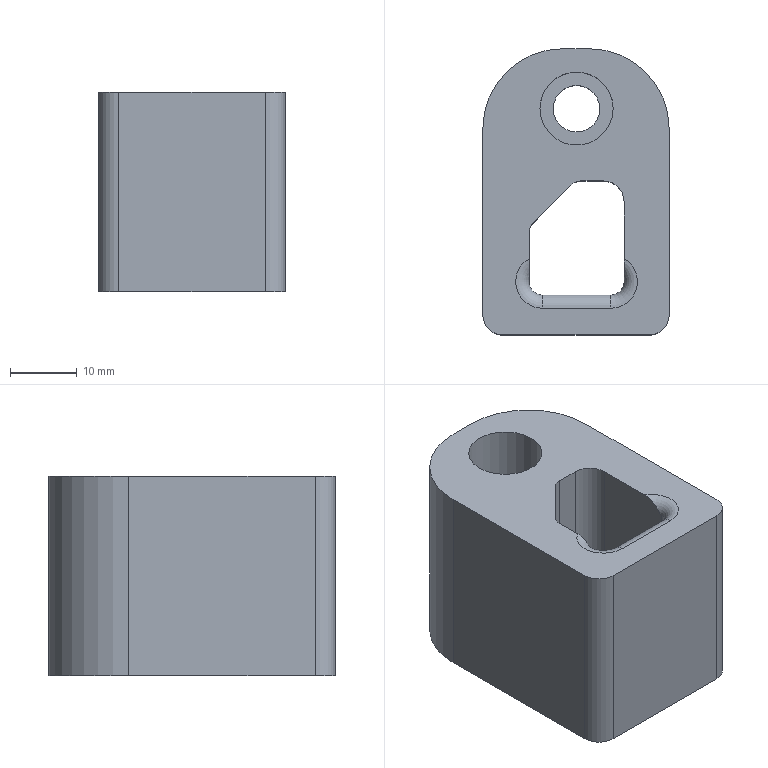Part | STEP file | 1 solid | 26 faces | box 28 x 43 x 30 mm | volume 25680 mm3 | plane 12 | cylinder 11 | torus 2 | spline 1 | commonest cylinder face diameters 4 x3 6 x2 24 x2 4.28 x1 6.28 x1 7 x1
STEP:
#1=CARTESIAN_POINT('',(-205.,-85.,-32.));
#2=VERTEX_POINT('',#1);
#3=CARTESIAN_POINT('',(-201.5,-85.,-32.));
#4=DIRECTION('',(0.,0.,-1.));
#5=DIRECTION('',(-1.,0.,0.));
#6=AXIS2_PLACEMENT_3D('',#3,#4,#5);
#7=CIRCLE('',#6,3.5);
#8=EDGE_CURVE('',#2,#2,#7,.T.);
#9=ORIENTED_EDGE('',*,*,#8,.F.);
#10=EDGE_LOOP('',(#9));
#11=FACE_BOUND('',#10,.T.);
#12=CARTESIAN_POINT('',(-212.586,-119.,-32.));
#13=VERTEX_POINT('',#12);
#14=CARTESIAN_POINT('',(-190.586,-119.,-32.));
#15=VERTEX_POINT('',#14);
#16=CARTESIAN_POINT('',(-200.586,-119.,-32.));
#17=DIRECTION('',(1.,0.,0.));
#18=VECTOR('',#17,1.);
#19=LINE('',#16,#18);
#20=EDGE_CURVE('',#13,#15,#19,.T.);
#21=ORIENTED_EDGE('',*,*,#20,.F.);
#22=CARTESIAN_POINT('',(-215.586,-116.,-32.));
#23=VERTEX_POINT('',#22);
#24=CARTESIAN_POINT('',(-212.586,-116.,-32.));
#25=DIRECTION('',(0.,0.,-1.));
#26=DIRECTION('',(-1.,0.,0.));
#27=AXIS2_PLACEMENT_3D('',#24,#25,#26);
#28=CIRCLE('',#27,3.);
#29=EDGE_CURVE('',#13,#23,#28,.T.);
#30=ORIENTED_EDGE('',*,*,#29,.T.);
#31=CARTESIAN_POINT('',(-215.586,-88.,-32.));
#32=VERTEX_POINT('',#31);
#33=CARTESIAN_POINT('',(-215.586,-98.5,-32.));
#34=DIRECTION('',(0.,-1.,0.));
#35=VECTOR('',#34,1.);
#36=LINE('',#33,#35);
#37=EDGE_CURVE('',#32,#23,#36,.T.);
#38=ORIENTED_EDGE('',*,*,#37,.F.);
#39=CARTESIAN_POINT('',(-203.586,-76.,-32.));
#40=VERTEX_POINT('',#39);
#41=CARTESIAN_POINT('',(-203.586,-88.,-32.));
#42=DIRECTION('',(0.,0.,-1.));
#43=DIRECTION('',(-1.,0.,0.));
#44=AXIS2_PLACEMENT_3D('',#41,#42,#43);
#45=CIRCLE('',#44,12.);
#46=EDGE_CURVE('',#32,#40,#45,.T.);
#47=ORIENTED_EDGE('',*,*,#46,.T.);
#48=CARTESIAN_POINT('',(-199.586,-76.,-32.));
#49=VERTEX_POINT('',#48);
#50=CARTESIAN_POINT('',(-200.586,-76.,-32.));
#51=DIRECTION('',(-1.,0.,0.));
#52=VECTOR('',#51,1.);
#53=LINE('',#50,#52);
#54=EDGE_CURVE('',#49,#40,#53,.T.);
#55=ORIENTED_EDGE('',*,*,#54,.F.);
#56=CARTESIAN_POINT('',(-187.586,-88.,-32.));
#57=VERTEX_POINT('',#56);
#58=CARTESIAN_POINT('',(-199.586,-88.,-32.));
#59=DIRECTION('',(0.,0.,-1.));
#60=DIRECTION('',(-1.,0.,0.));
#61=AXIS2_PLACEMENT_3D('',#58,#59,#60);
#62=CIRCLE('',#61,12.);
#63=EDGE_CURVE('',#49,#57,#62,.T.);
#64=ORIENTED_EDGE('',*,*,#63,.T.);
#65=CARTESIAN_POINT('',(-187.586,-116.,-32.));
#66=VERTEX_POINT('',#65);
#67=CARTESIAN_POINT('',(-187.586,-98.5,-32.));
#68=DIRECTION('',(0.,1.,0.));
#69=VECTOR('',#68,1.);
#70=LINE('',#67,#69);
#71=EDGE_CURVE('',#66,#57,#70,.T.);
#72=ORIENTED_EDGE('',*,*,#71,.F.);
#73=CARTESIAN_POINT('',(-190.586,-116.,-32.));
#74=DIRECTION('',(0.,0.,-1.));
#75=DIRECTION('',(-1.,0.,0.));
#76=AXIS2_PLACEMENT_3D('',#73,#74,#75);
#77=CIRCLE('',#76,3.);
#78=EDGE_CURVE('',#66,#15,#77,.T.);
#79=ORIENTED_EDGE('',*,*,#78,.T.);
#80=EDGE_LOOP('',(#21,#30,#38,#47,#55,#64,#72,#79));
#81=FACE_BOUND('',#80,.T.);
#82=CARTESIAN_POINT('',(-200.843,-95.86,-32.));
#83=VERTEX_POINT('',#82);
#84=CARTESIAN_POINT('',(-202.356,-96.487,-32.));
#85=VERTEX_POINT('',#84);
#86=CARTESIAN_POINT('',(-200.843,-95.86,-32.));
#87=CARTESIAN_POINT('',(-200.984,-95.86,-32.));
#88=CARTESIAN_POINT('',(-201.126,-95.874,-32.));
#89=CARTESIAN_POINT('',(-201.264,-95.901,-32.));
#90=CARTESIAN_POINT('',(-201.499,-95.949,-32.));
#91=CARTESIAN_POINT('',(-201.729,-96.037,-32.));
#92=CARTESIAN_POINT('',(-201.935,-96.159,-32.));
#93=CARTESIAN_POINT('',(-202.088,-96.25,-32.));
#94=CARTESIAN_POINT('',(-202.231,-96.361,-32.));
#95=CARTESIAN_POINT('',(-202.356,-96.487,-32.));
#96=B_SPLINE_CURVE_WITH_KNOTS('',3,(#86,#87,#88,#89,#90,#91,#92,#93,#94,#95),.UNSPECIFIED.,.F.,.F.,(4,3,3,4),(0.,0.2513,0.6822,1.),.UNSPECIFIED.);
#97=EDGE_CURVE('',#83,#85,#96,.T.);
#98=ORIENTED_EDGE('',*,*,#97,.T.);
#99=CARTESIAN_POINT('',(-208.013,-102.144,-32.));
#100=VERTEX_POINT('',#99);
#101=CARTESIAN_POINT('',(-206.771,-100.901,-32.));
#102=DIRECTION('',(-0.7071,-0.7071,0.));
#103=VECTOR('',#102,1.);
#104=LINE('',#101,#103);
#105=EDGE_CURVE('',#85,#100,#104,.T.);
#106=ORIENTED_EDGE('',*,*,#105,.T.);
#107=CARTESIAN_POINT('',(-208.64,-103.657,-32.));
#108=VERTEX_POINT('',#107);
#109=CARTESIAN_POINT('',(-206.5,-103.657,-32.));
#110=DIRECTION('',(0.,0.,1.));
#111=DIRECTION('',(-1.,0.,0.));
#112=AXIS2_PLACEMENT_3D('',#109,#110,#111);
#113=CIRCLE('',#112,2.14);
#114=EDGE_CURVE('',#100,#108,#113,.T.);
#115=ORIENTED_EDGE('',*,*,#114,.T.);
#116=CARTESIAN_POINT('',(-208.64,-111.,-32.));
#117=VERTEX_POINT('',#116);
#118=CARTESIAN_POINT('',(-208.64,-104.5,-32.));
#119=DIRECTION('',(0.,1.,0.));
#120=VECTOR('',#119,1.);
#121=LINE('',#118,#120);
#122=EDGE_CURVE('',#117,#108,#121,.T.);
#123=ORIENTED_EDGE('',*,*,#122,.F.);
#124=CARTESIAN_POINT('',(-206.64,-113.,-32.));
#125=VERTEX_POINT('',#124);
#126=CARTESIAN_POINT('',(-206.64,-111.,-32.));
#127=DIRECTION('',(0.,0.,1.));
#128=DIRECTION('',(-1.,0.,0.));
#129=AXIS2_PLACEMENT_3D('',#126,#127,#128);
#130=CIRCLE('',#129,2.);
#131=EDGE_CURVE('',#117,#125,#130,.T.);
#132=ORIENTED_EDGE('',*,*,#131,.T.);
#133=CARTESIAN_POINT('',(-196.36,-113.,-32.));
#134=VERTEX_POINT('',#133);
#135=CARTESIAN_POINT('',(-194.5,-113.,-32.));
#136=DIRECTION('',(1.,0.,0.));
#137=VECTOR('',#136,1.);
#138=LINE('',#135,#137);
#139=EDGE_CURVE('',#125,#134,#138,.T.);
#140=ORIENTED_EDGE('',*,*,#139,.T.);
#141=CARTESIAN_POINT('',(-194.36,-111.,-32.));
#142=VERTEX_POINT('',#141);
#143=CARTESIAN_POINT('',(-196.36,-111.,-32.));
#144=DIRECTION('',(0.,0.,1.));
#145=DIRECTION('',(-1.,0.,0.));
#146=AXIS2_PLACEMENT_3D('',#143,#144,#145);
#147=CIRCLE('',#146,2.);
#148=EDGE_CURVE('',#134,#142,#147,.T.);
#149=ORIENTED_EDGE('',*,*,#148,.T.);
#150=CARTESIAN_POINT('',(-194.36,-99.,-32.));
#151=VERTEX_POINT('',#150);
#152=CARTESIAN_POINT('',(-194.36,-99.,-32.));
#153=DIRECTION('',(0.,1.,0.));
#154=VECTOR('',#153,1.);
#155=LINE('',#152,#154);
#156=EDGE_CURVE('',#142,#151,#155,.T.);
#157=ORIENTED_EDGE('',*,*,#156,.T.);
#158=CARTESIAN_POINT('',(-197.5,-95.86,-32.));
#159=VERTEX_POINT('',#158);
#160=CARTESIAN_POINT('',(-197.5,-99.,-32.));
#161=DIRECTION('',(0.,0.,1.));
#162=DIRECTION('',(-1.,0.,0.));
#163=AXIS2_PLACEMENT_3D('',#160,#161,#162);
#164=CIRCLE('',#163,3.14);
#165=EDGE_CURVE('',#151,#159,#164,.T.);
#166=ORIENTED_EDGE('',*,*,#165,.T.);
#167=CARTESIAN_POINT('',(-200.843,-95.86,-32.));
#168=DIRECTION('',(-1.,0.,0.));
#169=VECTOR('',#168,1.);
#170=LINE('',#167,#169);
#171=EDGE_CURVE('',#159,#83,#170,.T.);
#172=ORIENTED_EDGE('',*,*,#171,.T.);
#173=EDGE_LOOP('',(#98,#106,#115,#123,#132,#140,#149,#157,#166,#172));
#174=FACE_BOUND('',#173,.T.);
#175=CARTESIAN_POINT('',(-201.5,-9.5,-32.));
#176=DIRECTION('',(0.,0.,-1.));
#177=DIRECTION('',(-1.,0.,0.));
#178=AXIS2_PLACEMENT_3D('',#175,#176,#177);
#179=PLANE('',#178);
#180=ADVANCED_FACE('',(#11,#81,#174),#179,.T.);
#181=CARTESIAN_POINT('',(-196.,-85.,-2.));
#182=VERTEX_POINT('',#181);
#183=CARTESIAN_POINT('',(-201.5,-85.,-2.));
#184=DIRECTION('',(0.,0.,-1.));
#185=DIRECTION('',(1.,0.,0.));
#186=AXIS2_PLACEMENT_3D('',#183,#184,#185);
#187=CIRCLE('',#186,5.5);
#188=EDGE_CURVE('',#182,#182,#187,.T.);
#189=ORIENTED_EDGE('',*,*,#188,.T.);
#190=EDGE_LOOP('',(#189));
#191=FACE_BOUND('',#190,.T.);
#192=CARTESIAN_POINT('',(-194.36,-107.536,-2.));
#193=VERTEX_POINT('',#192);
#194=CARTESIAN_POINT('',(-194.36,-99.,-2.));
#195=VERTEX_POINT('',#194);
#196=CARTESIAN_POINT('',(-194.36,129.,-2.));
#197=DIRECTION('',(0.,1.,0.));
#198=VECTOR('',#197,1.);
#199=LINE('',#196,#198);
#200=EDGE_CURVE('',#193,#195,#199,.T.);
#201=ORIENTED_EDGE('',*,*,#200,.F.);
#202=CARTESIAN_POINT('',(-196.36,-115.,-2.));
#203=VERTEX_POINT('',#202);
#204=CARTESIAN_POINT('',(-196.36,-111.,-2.));
#205=DIRECTION('',(0.,0.,-1.));
#206=DIRECTION('',(1.,0.,0.));
#207=AXIS2_PLACEMENT_3D('',#204,#205,#206);
#208=CIRCLE('',#207,4.);
#209=EDGE_CURVE('',#193,#203,#208,.T.);
#210=ORIENTED_EDGE('',*,*,#209,.T.);
#211=CARTESIAN_POINT('',(-206.64,-115.,-2.));
#212=VERTEX_POINT('',#211);
#213=CARTESIAN_POINT('',(-206.64,-115.,-2.));
#214=DIRECTION('',(-1.,0.,0.));
#215=VECTOR('',#214,1.);
#216=LINE('',#213,#215);
#217=EDGE_CURVE('',#203,#212,#216,.T.);
#218=ORIENTED_EDGE('',*,*,#217,.T.);
#219=CARTESIAN_POINT('',(-208.64,-107.536,-2.));
#220=VERTEX_POINT('',#219);
#221=CARTESIAN_POINT('',(-206.64,-111.,-2.));
#222=DIRECTION('',(0.,0.,-1.));
#223=DIRECTION('',(1.,0.,0.));
#224=AXIS2_PLACEMENT_3D('',#221,#222,#223);
#225=CIRCLE('',#224,4.);
#226=EDGE_CURVE('',#212,#220,#225,.T.);
#227=ORIENTED_EDGE('',*,*,#226,.T.);
#228=CARTESIAN_POINT('',(-208.64,-103.657,-2.));
#229=VERTEX_POINT('',#228);
#230=CARTESIAN_POINT('',(-208.64,129.,-2.));
#231=DIRECTION('',(0.,1.,0.));
#232=VECTOR('',#231,1.);
#233=LINE('',#230,#232);
#234=EDGE_CURVE('',#220,#229,#233,.T.);
#235=ORIENTED_EDGE('',*,*,#234,.T.);
#236=CARTESIAN_POINT('',(-208.013,-102.144,-2.));
#237=VERTEX_POINT('',#236);
#238=CARTESIAN_POINT('',(-206.5,-103.657,-2.));
#239=DIRECTION('',(0.,0.,1.));
#240=DIRECTION('',(1.,0.,0.));
#241=AXIS2_PLACEMENT_3D('',#238,#239,#240);
#242=CIRCLE('',#241,2.14);
#243=EDGE_CURVE('',#237,#229,#242,.T.);
#244=ORIENTED_EDGE('',*,*,#243,.F.);
#245=CARTESIAN_POINT('',(-202.356,-96.487,-2.));
#246=VERTEX_POINT('',#245);
#247=CARTESIAN_POINT('',(-128.91,-23.041,-2.));
#248=DIRECTION('',(-0.7071,-0.7071,0.));
#249=VECTOR('',#248,1.);
#250=LINE('',#247,#249);
#251=EDGE_CURVE('',#246,#237,#250,.T.);
#252=ORIENTED_EDGE('',*,*,#251,.F.);
#253=CARTESIAN_POINT('',(-200.843,-95.86,-2.));
#254=VERTEX_POINT('',#253);
#255=CARTESIAN_POINT('',(-200.843,-95.86,-2.));
#256=CARTESIAN_POINT('',(-200.984,-95.86,-2.));
#257=CARTESIAN_POINT('',(-201.126,-95.874,-2.));
#258=CARTESIAN_POINT('',(-201.264,-95.901,-2.));
#259=CARTESIAN_POINT('',(-201.499,-95.949,-2.));
#260=CARTESIAN_POINT('',(-201.729,-96.037,-2.));
#261=CARTESIAN_POINT('',(-201.935,-96.159,-2.));
#262=CARTESIAN_POINT('',(-202.088,-96.25,-2.));
#263=CARTESIAN_POINT('',(-202.231,-96.361,-2.));
#264=CARTESIAN_POINT('',(-202.356,-96.487,-2.));
#265=B_SPLINE_CURVE_WITH_KNOTS('',3,(#255,#256,#257,#258,#259,#260,#261,#262,#263,#264),.UNSPECIFIED.,.F.,.F.,(4,3,3,4),(0.,0.2513,0.6822,1.),.UNSPECIFIED.);
#266=EDGE_CURVE('',#254,#246,#265,.T.);
#267=ORIENTED_EDGE('',*,*,#266,.F.);
#268=CARTESIAN_POINT('',(-197.5,-95.86,-2.));
#269=VERTEX_POINT('',#268);
#270=CARTESIAN_POINT('',(-280.951,-95.86,-2.));
#271=DIRECTION('',(-1.,0.,0.));
#272=VECTOR('',#271,1.);
#273=LINE('',#270,#272);
#274=EDGE_CURVE('',#269,#254,#273,.T.);
#275=ORIENTED_EDGE('',*,*,#274,.F.);
#276=CARTESIAN_POINT('',(-197.5,-99.,-2.));
#277=DIRECTION('',(0.,0.,-1.));
#278=DIRECTION('',(1.,0.,0.));
#279=AXIS2_PLACEMENT_3D('',#276,#277,#278);
#280=CIRCLE('',#279,3.14);
#281=EDGE_CURVE('',#269,#195,#280,.T.);
#282=ORIENTED_EDGE('',*,*,#281,.T.);
#283=EDGE_LOOP('',(#201,#210,#218,#227,#235,#244,#252,#267,#275,#282));
#284=FACE_BOUND('',#283,.T.);
#285=CARTESIAN_POINT('',(-215.586,-116.,-2.));
#286=VERTEX_POINT('',#285);
#287=CARTESIAN_POINT('',(-215.586,-88.,-2.));
#288=VERTEX_POINT('',#287);
#289=CARTESIAN_POINT('',(-215.586,-98.5,-2.));
#290=DIRECTION('',(0.,1.,0.));
#291=VECTOR('',#290,1.);
#292=LINE('',#289,#291);
#293=EDGE_CURVE('',#286,#288,#292,.T.);
#294=ORIENTED_EDGE('',*,*,#293,.F.);
#295=CARTESIAN_POINT('',(-212.586,-119.,-2.));
#296=VERTEX_POINT('',#295);
#297=CARTESIAN_POINT('',(-212.586,-116.,-2.));
#298=DIRECTION('',(0.,0.,1.));
#299=DIRECTION('',(1.,0.,0.));
#300=AXIS2_PLACEMENT_3D('',#297,#298,#299);
#301=CIRCLE('',#300,3.);
#302=EDGE_CURVE('',#286,#296,#301,.T.);
#303=ORIENTED_EDGE('',*,*,#302,.T.);
#304=CARTESIAN_POINT('',(-190.586,-119.,-2.));
#305=VERTEX_POINT('',#304);
#306=CARTESIAN_POINT('',(-200.586,-119.,-2.));
#307=DIRECTION('',(-1.,0.,0.));
#308=VECTOR('',#307,1.);
#309=LINE('',#306,#308);
#310=EDGE_CURVE('',#305,#296,#309,.T.);
#311=ORIENTED_EDGE('',*,*,#310,.F.);
#312=CARTESIAN_POINT('',(-187.586,-116.,-2.));
#313=VERTEX_POINT('',#312);
#314=CARTESIAN_POINT('',(-190.586,-116.,-2.));
#315=DIRECTION('',(0.,0.,1.));
#316=DIRECTION('',(1.,0.,0.));
#317=AXIS2_PLACEMENT_3D('',#314,#315,#316);
#318=CIRCLE('',#317,3.);
#319=EDGE_CURVE('',#305,#313,#318,.T.);
#320=ORIENTED_EDGE('',*,*,#319,.T.);
#321=CARTESIAN_POINT('',(-187.586,-88.,-2.));
#322=VERTEX_POINT('',#321);
#323=CARTESIAN_POINT('',(-187.586,-98.5,-2.));
#324=DIRECTION('',(0.,-1.,0.));
#325=VECTOR('',#324,1.);
#326=LINE('',#323,#325);
#327=EDGE_CURVE('',#322,#313,#326,.T.);
#328=ORIENTED_EDGE('',*,*,#327,.F.);
#329=CARTESIAN_POINT('',(-199.586,-76.,-2.));
#330=VERTEX_POINT('',#329);
#331=CARTESIAN_POINT('',(-199.586,-88.,-2.));
#332=DIRECTION('',(0.,0.,1.));
#333=DIRECTION('',(1.,0.,0.));
#334=AXIS2_PLACEMENT_3D('',#331,#332,#333);
#335=CIRCLE('',#334,12.);
#336=EDGE_CURVE('',#322,#330,#335,.T.);
#337=ORIENTED_EDGE('',*,*,#336,.T.);
#338=CARTESIAN_POINT('',(-203.586,-76.,-2.));
#339=VERTEX_POINT('',#338);
#340=CARTESIAN_POINT('',(-200.586,-76.,-2.));
#341=DIRECTION('',(1.,0.,0.));
#342=VECTOR('',#341,1.);
#343=LINE('',#340,#342);
#344=EDGE_CURVE('',#339,#330,#343,.T.);
#345=ORIENTED_EDGE('',*,*,#344,.F.);
#346=CARTESIAN_POINT('',(-203.586,-88.,-2.));
#347=DIRECTION('',(0.,0.,1.));
#348=DIRECTION('',(1.,0.,0.));
#349=AXIS2_PLACEMENT_3D('',#346,#347,#348);
#350=CIRCLE('',#349,12.);
#351=EDGE_CURVE('',#339,#288,#350,.T.);
#352=ORIENTED_EDGE('',*,*,#351,.T.);
#353=EDGE_LOOP('',(#294,#303,#311,#320,#328,#337,#345,#352));
#354=FACE_BOUND('',#353,.T.);
#355=CARTESIAN_POINT('',(-280.951,129.,-2.));
#356=DIRECTION('',(0.,0.,1.));
#357=DIRECTION('',(1.,0.,0.));
#358=AXIS2_PLACEMENT_3D('',#355,#356,#357);
#359=PLANE('',#358);
#360=ADVANCED_FACE('',(#191,#284,#354),#359,.T.);
#361=ORIENTED_EDGE('',*,*,#310,.T.);
#362=CARTESIAN_POINT('',(-212.586,-119.,-2.));
#363=DIRECTION('',(0.,0.,-1.));
#364=VECTOR('',#363,1.);
#365=LINE('',#362,#364);
#366=EDGE_CURVE('',#296,#13,#365,.T.);
#367=ORIENTED_EDGE('',*,*,#366,.T.);
#368=ORIENTED_EDGE('',*,*,#20,.T.);
#369=CARTESIAN_POINT('',(-190.586,-119.,-2.));
#370=DIRECTION('',(0.,0.,1.));
#371=VECTOR('',#370,1.);
#372=LINE('',#369,#371);
#373=EDGE_CURVE('',#15,#305,#372,.T.);
#374=ORIENTED_EDGE('',*,*,#373,.T.);
#375=EDGE_LOOP('',(#361,#367,#368,#374));
#376=FACE_OUTER_BOUND('',#375,.T.);
#377=CARTESIAN_POINT('',(-200.586,-119.,-2.));
#378=DIRECTION('',(0.,-1.,0.));
#379=DIRECTION('',(0.,0.,-1.));
#380=AXIS2_PLACEMENT_3D('',#377,#378,#379);
#381=PLANE('',#380);
#382=ADVANCED_FACE('',(#376),#381,.T.);
#383=ORIENTED_EDGE('',*,*,#37,.T.);
#384=CARTESIAN_POINT('',(-215.586,-116.,-2.));
#385=DIRECTION('',(0.,0.,1.));
#386=VECTOR('',#385,1.);
#387=LINE('',#384,#386);
#388=EDGE_CURVE('',#23,#286,#387,.T.);
#389=ORIENTED_EDGE('',*,*,#388,.T.);
#390=ORIENTED_EDGE('',*,*,#293,.T.);
#391=CARTESIAN_POINT('',(-215.586,-88.,-2.));
#392=DIRECTION('',(0.,0.,-1.));
#393=VECTOR('',#392,1.);
#394=LINE('',#391,#393);
#395=EDGE_CURVE('',#288,#32,#394,.T.);
#396=ORIENTED_EDGE('',*,*,#395,.T.);
#397=EDGE_LOOP('',(#383,#389,#390,#396));
#398=FACE_OUTER_BOUND('',#397,.T.);
#399=CARTESIAN_POINT('',(-215.586,-98.5,-2.));
#400=DIRECTION('',(-1.,0.,0.));
#401=DIRECTION('',(0.,0.,1.));
#402=AXIS2_PLACEMENT_3D('',#399,#400,#401);
#403=PLANE('',#402);
#404=ADVANCED_FACE('',(#398),#403,.T.);
#405=ORIENTED_EDGE('',*,*,#344,.T.);
#406=CARTESIAN_POINT('',(-199.586,-76.,-2.));
#407=DIRECTION('',(0.,0.,-1.));
#408=VECTOR('',#407,1.);
#409=LINE('',#406,#408);
#410=EDGE_CURVE('',#330,#49,#409,.T.);
#411=ORIENTED_EDGE('',*,*,#410,.T.);
#412=ORIENTED_EDGE('',*,*,#54,.T.);
#413=CARTESIAN_POINT('',(-203.586,-76.,-2.));
#414=DIRECTION('',(0.,0.,1.));
#415=VECTOR('',#414,1.);
#416=LINE('',#413,#415);
#417=EDGE_CURVE('',#40,#339,#416,.T.);
#418=ORIENTED_EDGE('',*,*,#417,.T.);
#419=EDGE_LOOP('',(#405,#411,#412,#418));
#420=FACE_OUTER_BOUND('',#419,.T.);
#421=CARTESIAN_POINT('',(-200.586,-76.,-2.));
#422=DIRECTION('',(0.,1.,0.));
#423=DIRECTION('',(0.,0.,1.));
#424=AXIS2_PLACEMENT_3D('',#421,#422,#423);
#425=PLANE('',#424);
#426=ADVANCED_FACE('',(#420),#425,.T.);
#427=ORIENTED_EDGE('',*,*,#327,.T.);
#428=CARTESIAN_POINT('',(-187.586,-116.,-2.));
#429=DIRECTION('',(0.,0.,-1.));
#430=VECTOR('',#429,1.);
#431=LINE('',#428,#430);
#432=EDGE_CURVE('',#313,#66,#431,.T.);
#433=ORIENTED_EDGE('',*,*,#432,.T.);
#434=ORIENTED_EDGE('',*,*,#71,.T.);
#435=CARTESIAN_POINT('',(-187.586,-88.,-2.));
#436=DIRECTION('',(0.,0.,1.));
#437=VECTOR('',#436,1.);
#438=LINE('',#435,#437);
#439=EDGE_CURVE('',#57,#322,#438,.T.);
#440=ORIENTED_EDGE('',*,*,#439,.T.);
#441=EDGE_LOOP('',(#427,#433,#434,#440));
#442=FACE_OUTER_BOUND('',#441,.T.);
#443=CARTESIAN_POINT('',(-187.586,-98.5,-2.));
#444=DIRECTION('',(1.,0.,0.));
#445=DIRECTION('',(0.,0.,-1.));
#446=AXIS2_PLACEMENT_3D('',#443,#444,#445);
#447=PLANE('',#446);
#448=ADVANCED_FACE('',(#442),#447,.T.);
#449=CARTESIAN_POINT('',(-206.64,-113.,-4.));
#450=VERTEX_POINT('',#449);
#451=CARTESIAN_POINT('',(-206.64,-113.,28.));
#452=DIRECTION('',(0.,0.,1.));
#453=VECTOR('',#452,1.);
#454=LINE('',#451,#453);
#455=EDGE_CURVE('',#125,#450,#454,.T.);
#456=ORIENTED_EDGE('',*,*,#455,.T.);
#457=CARTESIAN_POINT('',(-196.36,-113.,-4.));
#458=VERTEX_POINT('',#457);
#459=CARTESIAN_POINT('',(-196.36,-113.,-4.));
#460=DIRECTION('',(1.,0.,0.));
#461=VECTOR('',#460,1.);
#462=LINE('',#459,#461);
#463=EDGE_CURVE('',#450,#458,#462,.T.);
#464=ORIENTED_EDGE('',*,*,#463,.T.);
#465=CARTESIAN_POINT('',(-196.36,-113.,-32.));
#466=DIRECTION('',(0.,0.,-1.));
#467=VECTOR('',#466,1.);
#468=LINE('',#465,#467);
#469=EDGE_CURVE('',#458,#134,#468,.T.);
#470=ORIENTED_EDGE('',*,*,#469,.T.);
#471=ORIENTED_EDGE('',*,*,#139,.F.);
#472=EDGE_LOOP('',(#456,#464,#470,#471));
#473=FACE_OUTER_BOUND('',#472,.T.);
#474=CARTESIAN_POINT('',(-194.5,-113.,28.));
#475=DIRECTION('',(0.,-1.,0.));
#476=DIRECTION('',(0.,0.,-1.));
#477=AXIS2_PLACEMENT_3D('',#474,#475,#476);
#478=PLANE('',#477);
#479=ADVANCED_FACE('',(#473),#478,.F.);
#480=ORIENTED_EDGE('',*,*,#234,.F.);
#481=CARTESIAN_POINT('',(-208.64,-111.,-4.));
#482=VERTEX_POINT('',#481);
#483=CARTESIAN_POINT('',(-208.64,-107.536,-2.));
#484=CARTESIAN_POINT('',(-208.64,-107.875,-2.));
#485=CARTESIAN_POINT('',(-208.64,-108.217,-2.066));
#486=CARTESIAN_POINT('',(-208.64,-108.536,-2.179));
#487=CARTESIAN_POINT('',(-208.64,-108.973,-2.333));
#488=CARTESIAN_POINT('',(-208.64,-109.381,-2.576));
#489=CARTESIAN_POINT('',(-208.64,-109.749,-2.857));
#490=CARTESIAN_POINT('',(-208.64,-110.196,-3.197));
#491=CARTESIAN_POINT('',(-208.64,-110.596,-3.596));
#492=CARTESIAN_POINT('',(-208.64,-110.994,-3.994));
#493=CARTESIAN_POINT('',(-208.64,-110.996,-3.996));
#494=CARTESIAN_POINT('',(-208.64,-110.998,-3.998));
#495=CARTESIAN_POINT('',(-208.64,-111.,-4.));
#496=B_SPLINE_CURVE_WITH_KNOTS('',3,(#483,#484,#485,#486,#487,#488,#489,#490,#491,#492,#493,#494,#495),.UNSPECIFIED.,.F.,.F.,(4,3,3,3,4),(0.,0.2481,0.588,0.9978,1.),.UNSPECIFIED.);
#497=EDGE_CURVE('',#220,#482,#496,.T.);
#498=ORIENTED_EDGE('',*,*,#497,.T.);
#499=CARTESIAN_POINT('',(-208.64,-111.,13.));
#500=DIRECTION('',(0.,0.,-1.));
#501=VECTOR('',#500,1.);
#502=LINE('',#499,#501);
#503=EDGE_CURVE('',#482,#117,#502,.T.);
#504=ORIENTED_EDGE('',*,*,#503,.T.);
#505=ORIENTED_EDGE('',*,*,#122,.T.);
#506=CARTESIAN_POINT('',(-208.64,-103.657,13.));
#507=DIRECTION('',(0.,0.,1.));
#508=VECTOR('',#507,1.);
#509=LINE('',#506,#508);
#510=EDGE_CURVE('',#108,#229,#509,.T.);
#511=ORIENTED_EDGE('',*,*,#510,.T.);
#512=EDGE_LOOP('',(#480,#498,#504,#505,#511));
#513=FACE_OUTER_BOUND('',#512,.T.);
#514=CARTESIAN_POINT('',(-208.64,-104.5,13.));
#515=DIRECTION('',(1.,0.,0.));
#516=DIRECTION('',(0.,0.,-1.));
#517=AXIS2_PLACEMENT_3D('',#514,#515,#516);
#518=PLANE('',#517);
#519=ADVANCED_FACE('',(#513),#518,.T.);
#520=CARTESIAN_POINT('',(-194.36,-111.,-4.));
#521=VERTEX_POINT('',#520);
#522=CARTESIAN_POINT('',(-194.36,-111.,-2.));
#523=DIRECTION('',(0.,0.,1.));
#524=VECTOR('',#523,1.);
#525=LINE('',#522,#524);
#526=EDGE_CURVE('',#142,#521,#525,.T.);
#527=ORIENTED_EDGE('',*,*,#526,.T.);
#528=CARTESIAN_POINT('',(-194.36,-111.,-4.));
#529=CARTESIAN_POINT('',(-194.36,-110.998,-3.998));
#530=CARTESIAN_POINT('',(-194.36,-110.996,-3.996));
#531=CARTESIAN_POINT('',(-194.36,-110.994,-3.994));
#532=CARTESIAN_POINT('',(-194.36,-110.596,-3.596));
#533=CARTESIAN_POINT('',(-194.36,-110.196,-3.197));
#534=CARTESIAN_POINT('',(-194.36,-109.749,-2.857));
#535=CARTESIAN_POINT('',(-194.36,-109.381,-2.576));
#536=CARTESIAN_POINT('',(-194.36,-108.973,-2.333));
#537=CARTESIAN_POINT('',(-194.36,-108.536,-2.179));
#538=CARTESIAN_POINT('',(-194.36,-108.217,-2.066));
#539=CARTESIAN_POINT('',(-194.36,-107.875,-2.));
#540=CARTESIAN_POINT('',(-194.36,-107.536,-2.));
#541=B_SPLINE_CURVE_WITH_KNOTS('',3,(#528,#529,#530,#531,#532,#533,#534,#535,#536,#537,#538,#539,#540),.UNSPECIFIED.,.F.,.F.,(4,3,3,3,4),(0.,0.002184,0.412,0.7519,1.),.UNSPECIFIED.);
#542=EDGE_CURVE('',#521,#193,#541,.T.);
#543=ORIENTED_EDGE('',*,*,#542,.T.);
#544=ORIENTED_EDGE('',*,*,#200,.T.);
#545=CARTESIAN_POINT('',(-194.36,-99.,28.));
#546=DIRECTION('',(0.,0.,-1.));
#547=VECTOR('',#546,1.);
#548=LINE('',#545,#547);
#549=EDGE_CURVE('',#195,#151,#548,.T.);
#550=ORIENTED_EDGE('',*,*,#549,.T.);
#551=ORIENTED_EDGE('',*,*,#156,.F.);
#552=EDGE_LOOP('',(#527,#543,#544,#550,#551));
#553=FACE_OUTER_BOUND('',#552,.T.);
#554=CARTESIAN_POINT('',(-194.36,-99.,28.));
#555=DIRECTION('',(1.,0.,0.));
#556=DIRECTION('',(0.,0.,-1.));
#557=AXIS2_PLACEMENT_3D('',#554,#555,#556);
#558=PLANE('',#557);
#559=ADVANCED_FACE('',(#553),#558,.F.);
#560=ORIENTED_EDGE('',*,*,#251,.T.);
#561=CARTESIAN_POINT('',(-208.013,-102.144,28.));
#562=DIRECTION('',(0.,0.,-1.));
#563=VECTOR('',#562,1.);
#564=LINE('',#561,#563);
#565=EDGE_CURVE('',#237,#100,#564,.T.);
#566=ORIENTED_EDGE('',*,*,#565,.T.);
#567=ORIENTED_EDGE('',*,*,#105,.F.);
#568=CARTESIAN_POINT('',(-202.356,-96.487,28.));
#569=DIRECTION('',(0.,0.,1.));
#570=VECTOR('',#569,1.);
#571=LINE('',#568,#570);
#572=EDGE_CURVE('',#85,#246,#571,.T.);
#573=ORIENTED_EDGE('',*,*,#572,.T.);
#574=EDGE_LOOP('',(#560,#566,#567,#573));
#575=FACE_OUTER_BOUND('',#574,.T.);
#576=CARTESIAN_POINT('',(-206.771,-100.901,28.));
#577=DIRECTION('',(-0.7071,0.7071,0.));
#578=DIRECTION('',(-0.7071,-0.7071,0.));
#579=AXIS2_PLACEMENT_3D('',#576,#577,#578);
#580=PLANE('',#579);
#581=ADVANCED_FACE('',(#575),#580,.F.);
#582=ORIENTED_EDGE('',*,*,#266,.T.);
#583=ORIENTED_EDGE('',*,*,#572,.F.);
#584=ORIENTED_EDGE('',*,*,#97,.F.);
#585=CARTESIAN_POINT('',(-200.843,-95.86,28.));
#586=DIRECTION('',(0.,0.,1.));
#587=VECTOR('',#586,1.);
#588=LINE('',#585,#587);
#589=EDGE_CURVE('',#83,#254,#588,.T.);
#590=ORIENTED_EDGE('',*,*,#589,.T.);
#591=EDGE_LOOP('',(#582,#583,#584,#590));
#592=FACE_OUTER_BOUND('',#591,.T.);
#593=CARTESIAN_POINT('',(-200.843,-95.86,-2.));
#594=CARTESIAN_POINT('',(-200.843,-95.86,-32.));
#595=CARTESIAN_POINT('',(-201.402,-95.86,-2.));
#596=CARTESIAN_POINT('',(-201.402,-95.86,-32.));
#597=CARTESIAN_POINT('',(-201.961,-96.091,-2.));
#598=CARTESIAN_POINT('',(-201.961,-96.091,-32.));
#599=CARTESIAN_POINT('',(-202.356,-96.487,-2.));
#600=CARTESIAN_POINT('',(-202.356,-96.487,-32.));
#601=B_SPLINE_SURFACE_WITH_KNOTS('',3,1,((#593,#594),(#595,#596),(#597,#598),(#599,#600)),.UNSPECIFIED.,.F.,.F.,.F.,(4,4),(2,2),(0.,1.),(0.,1.),.UNSPECIFIED.);
#602=ADVANCED_FACE('',(#592),#601,.T.);
#603=ORIENTED_EDGE('',*,*,#171,.F.);
#604=CARTESIAN_POINT('',(-197.5,-95.86,28.));
#605=DIRECTION('',(0.,0.,1.));
#606=VECTOR('',#605,1.);
#607=LINE('',#604,#606);
#608=EDGE_CURVE('',#159,#269,#607,.T.);
#609=ORIENTED_EDGE('',*,*,#608,.T.);
#610=ORIENTED_EDGE('',*,*,#274,.T.);
#611=ORIENTED_EDGE('',*,*,#589,.F.);
#612=EDGE_LOOP('',(#603,#609,#610,#611));
#613=FACE_OUTER_BOUND('',#612,.T.);
#614=CARTESIAN_POINT('',(-200.843,-95.86,28.));
#615=DIRECTION('',(0.,1.,0.));
#616=DIRECTION('',(0.,0.,1.));
#617=AXIS2_PLACEMENT_3D('',#614,#615,#616);
#618=PLANE('',#617);
#619=ADVANCED_FACE('',(#613),#618,.F.);
#620=ORIENTED_EDGE('',*,*,#243,.T.);
#621=ORIENTED_EDGE('',*,*,#510,.F.);
#622=ORIENTED_EDGE('',*,*,#114,.F.);
#623=ORIENTED_EDGE('',*,*,#565,.F.);
#624=EDGE_LOOP('',(#620,#621,#622,#623));
#625=FACE_OUTER_BOUND('',#624,.T.);
#626=CARTESIAN_POINT('',(-206.5,-103.657,13.));
#627=DIRECTION('',(0.,0.,1.));
#628=DIRECTION('',(1.,0.,0.));
#629=AXIS2_PLACEMENT_3D('',#626,#627,#628);
#630=CYLINDRICAL_SURFACE('',#629,2.14);
#631=ADVANCED_FACE('',(#625),#630,.F.);
#632=ORIENTED_EDGE('',*,*,#165,.F.);
#633=ORIENTED_EDGE('',*,*,#549,.F.);
#634=ORIENTED_EDGE('',*,*,#281,.F.);
#635=ORIENTED_EDGE('',*,*,#608,.F.);
#636=EDGE_LOOP('',(#632,#633,#634,#635));
#637=FACE_OUTER_BOUND('',#636,.T.);
#638=CARTESIAN_POINT('',(-197.5,-99.,28.));
#639=DIRECTION('',(0.,0.,-1.));
#640=DIRECTION('',(-1.,0.,0.));
#641=AXIS2_PLACEMENT_3D('',#638,#639,#640);
#642=CYLINDRICAL_SURFACE('',#641,3.14);
#643=ADVANCED_FACE('',(#637),#642,.F.);
#644=ORIENTED_EDGE('',*,*,#336,.F.);
#645=ORIENTED_EDGE('',*,*,#439,.F.);
#646=ORIENTED_EDGE('',*,*,#63,.F.);
#647=ORIENTED_EDGE('',*,*,#410,.F.);
#648=EDGE_LOOP('',(#644,#645,#646,#647));
#649=FACE_OUTER_BOUND('',#648,.T.);
#650=CARTESIAN_POINT('',(-199.586,-88.,-2.));
#651=DIRECTION('',(0.,0.,1.));
#652=DIRECTION('',(1.,0.,0.));
#653=AXIS2_PLACEMENT_3D('',#650,#651,#652);
#654=CYLINDRICAL_SURFACE('',#653,12.);
#655=ADVANCED_FACE('',(#649),#654,.T.);
#656=ORIENTED_EDGE('',*,*,#351,.F.);
#657=ORIENTED_EDGE('',*,*,#417,.F.);
#658=ORIENTED_EDGE('',*,*,#46,.F.);
#659=ORIENTED_EDGE('',*,*,#395,.F.);
#660=EDGE_LOOP('',(#656,#657,#658,#659));
#661=FACE_OUTER_BOUND('',#660,.T.);
#662=CARTESIAN_POINT('',(-203.586,-88.,-2.));
#663=DIRECTION('',(0.,0.,1.));
#664=DIRECTION('',(1.,0.,0.));
#665=AXIS2_PLACEMENT_3D('',#662,#663,#664);
#666=CYLINDRICAL_SURFACE('',#665,12.);
#667=ADVANCED_FACE('',(#661),#666,.T.);
#668=ORIENTED_EDGE('',*,*,#302,.F.);
#669=ORIENTED_EDGE('',*,*,#388,.F.);
#670=ORIENTED_EDGE('',*,*,#29,.F.);
#671=ORIENTED_EDGE('',*,*,#366,.F.);
#672=EDGE_LOOP('',(#668,#669,#670,#671));
#673=FACE_OUTER_BOUND('',#672,.T.);
#674=CARTESIAN_POINT('',(-212.586,-116.,-2.));
#675=DIRECTION('',(0.,0.,-1.));
#676=DIRECTION('',(-1.,0.,0.));
#677=AXIS2_PLACEMENT_3D('',#674,#675,#676);
#678=CYLINDRICAL_SURFACE('',#677,3.);
#679=ADVANCED_FACE('',(#673),#678,.T.);
#680=ORIENTED_EDGE('',*,*,#319,.F.);
#681=ORIENTED_EDGE('',*,*,#373,.F.);
#682=ORIENTED_EDGE('',*,*,#78,.F.);
#683=ORIENTED_EDGE('',*,*,#432,.F.);
#684=EDGE_LOOP('',(#680,#681,#682,#683));
#685=FACE_OUTER_BOUND('',#684,.T.);
#686=CARTESIAN_POINT('',(-190.586,-116.,-2.));
#687=DIRECTION('',(0.,0.,-1.));
#688=DIRECTION('',(-1.,0.,0.));
#689=AXIS2_PLACEMENT_3D('',#686,#687,#688);
#690=CYLINDRICAL_SURFACE('',#689,3.);
#691=ADVANCED_FACE('',(#685),#690,.T.);
#692=ORIENTED_EDGE('',*,*,#469,.F.);
#693=CARTESIAN_POINT('',(-196.36,-111.,-4.));
#694=DIRECTION('',(0.,0.,1.));
#695=DIRECTION('',(1.,0.,0.));
#696=AXIS2_PLACEMENT_3D('',#693,#694,#695);
#697=CIRCLE('',#696,2.);
#698=EDGE_CURVE('',#458,#521,#697,.T.);
#699=ORIENTED_EDGE('',*,*,#698,.T.);
#700=ORIENTED_EDGE('',*,*,#526,.F.);
#701=ORIENTED_EDGE('',*,*,#148,.F.);
#702=EDGE_LOOP('',(#692,#699,#700,#701));
#703=FACE_OUTER_BOUND('',#702,.T.);
#704=CARTESIAN_POINT('',(-196.36,-111.,28.));
#705=DIRECTION('',(0.,0.,-1.));
#706=DIRECTION('',(-1.,0.,0.));
#707=AXIS2_PLACEMENT_3D('',#704,#705,#706);
#708=CYLINDRICAL_SURFACE('',#707,2.);
#709=ADVANCED_FACE('',(#703),#708,.F.);
#710=ORIENTED_EDGE('',*,*,#503,.F.);
#711=CARTESIAN_POINT('',(-206.64,-111.,-4.));
#712=DIRECTION('',(0.,0.,1.));
#713=DIRECTION('',(1.,0.,0.));
#714=AXIS2_PLACEMENT_3D('',#711,#712,#713);
#715=CIRCLE('',#714,2.);
#716=EDGE_CURVE('',#482,#450,#715,.T.);
#717=ORIENTED_EDGE('',*,*,#716,.T.);
#718=ORIENTED_EDGE('',*,*,#455,.F.);
#719=ORIENTED_EDGE('',*,*,#131,.F.);
#720=EDGE_LOOP('',(#710,#717,#718,#719));
#721=FACE_OUTER_BOUND('',#720,.T.);
#722=CARTESIAN_POINT('',(-206.64,-111.,28.));
#723=DIRECTION('',(0.,0.,1.));
#724=DIRECTION('',(1.,0.,0.));
#725=AXIS2_PLACEMENT_3D('',#722,#723,#724);
#726=CYLINDRICAL_SURFACE('',#725,2.);
#727=ADVANCED_FACE('',(#721),#726,.F.);
#728=ORIENTED_EDGE('',*,*,#497,.F.);
#729=ORIENTED_EDGE('',*,*,#226,.F.);
#730=CARTESIAN_POINT('',(-206.64,-115.,-4.));
#731=DIRECTION('',(1.,0.,0.));
#732=DIRECTION('',(0.,0.,-1.));
#733=AXIS2_PLACEMENT_3D('',#730,#731,#732);
#734=CIRCLE('',#733,2.);
#735=EDGE_CURVE('',#450,#212,#734,.T.);
#736=ORIENTED_EDGE('',*,*,#735,.F.);
#737=ORIENTED_EDGE('',*,*,#716,.F.);
#738=EDGE_LOOP('',(#728,#729,#736,#737));
#739=FACE_OUTER_BOUND('',#738,.T.);
#740=CARTESIAN_POINT('',(-206.64,-111.,-4.));
#741=DIRECTION('',(0.,0.,1.));
#742=DIRECTION('',(1.,0.,0.));
#743=AXIS2_PLACEMENT_3D('',#740,#741,#742);
#744=TOROIDAL_SURFACE('',#743,4.,2.);
#745=ADVANCED_FACE('',(#739),#744,.T.);
#746=ORIENTED_EDGE('',*,*,#735,.T.);
#747=ORIENTED_EDGE('',*,*,#217,.F.);
#748=CARTESIAN_POINT('',(-196.36,-115.,-4.));
#749=DIRECTION('',(1.,0.,0.));
#750=DIRECTION('',(0.,0.,-1.));
#751=AXIS2_PLACEMENT_3D('',#748,#749,#750);
#752=CIRCLE('',#751,2.);
#753=EDGE_CURVE('',#458,#203,#752,.T.);
#754=ORIENTED_EDGE('',*,*,#753,.F.);
#755=ORIENTED_EDGE('',*,*,#463,.F.);
#756=EDGE_LOOP('',(#746,#747,#754,#755));
#757=FACE_OUTER_BOUND('',#756,.T.);
#758=CARTESIAN_POINT('',(-194.5,-115.,-4.));
#759=DIRECTION('',(-1.,0.,0.));
#760=DIRECTION('',(0.,0.,1.));
#761=AXIS2_PLACEMENT_3D('',#758,#759,#760);
#762=CYLINDRICAL_SURFACE('',#761,2.);
#763=ADVANCED_FACE('',(#757),#762,.T.);
#764=ORIENTED_EDGE('',*,*,#542,.F.);
#765=ORIENTED_EDGE('',*,*,#698,.F.);
#766=ORIENTED_EDGE('',*,*,#753,.T.);
#767=ORIENTED_EDGE('',*,*,#209,.F.);
#768=EDGE_LOOP('',(#764,#765,#766,#767));
#769=FACE_OUTER_BOUND('',#768,.T.);
#770=CARTESIAN_POINT('',(-196.36,-111.,-4.));
#771=DIRECTION('',(0.,0.,1.));
#772=DIRECTION('',(1.,0.,0.));
#773=AXIS2_PLACEMENT_3D('',#770,#771,#772);
#774=TOROIDAL_SURFACE('',#773,4.,2.);
#775=ADVANCED_FACE('',(#769),#774,.T.);
#776=ORIENTED_EDGE('',*,*,#8,.T.);
#777=EDGE_LOOP('',(#776));
#778=FACE_BOUND('',#777,.T.);
#779=CARTESIAN_POINT('',(-205.,-85.,-16.));
#780=VERTEX_POINT('',#779);
#781=CARTESIAN_POINT('',(-201.5,-85.,-16.));
#782=DIRECTION('',(0.,0.,-1.));
#783=DIRECTION('',(-1.,0.,0.));
#784=AXIS2_PLACEMENT_3D('',#781,#782,#783);
#785=CIRCLE('',#784,3.5);
#786=EDGE_CURVE('',#780,#780,#785,.T.);
#787=ORIENTED_EDGE('',*,*,#786,.F.);
#788=EDGE_LOOP('',(#787));
#789=FACE_BOUND('',#788,.T.);
#790=CARTESIAN_POINT('',(-201.5,-85.,-47.));
#791=DIRECTION('',(0.,0.,1.));
#792=DIRECTION('',(1.,0.,0.));
#793=AXIS2_PLACEMENT_3D('',#790,#791,#792);
#794=CYLINDRICAL_SURFACE('',#793,3.5);
#795=ADVANCED_FACE('',(#778,#789),#794,.F.);
#796=ORIENTED_EDGE('',*,*,#786,.T.);
#797=EDGE_LOOP('',(#796));
#798=FACE_BOUND('',#797,.T.);
#799=CARTESIAN_POINT('',(-196.,-85.,-16.));
#800=VERTEX_POINT('',#799);
#801=CARTESIAN_POINT('',(-201.5,-85.,-16.));
#802=DIRECTION('',(0.,0.,-1.));
#803=DIRECTION('',(1.,0.,0.));
#804=AXIS2_PLACEMENT_3D('',#801,#802,#803);
#805=CIRCLE('',#804,5.5);
#806=EDGE_CURVE('',#800,#800,#805,.T.);
#807=ORIENTED_EDGE('',*,*,#806,.F.);
#808=EDGE_LOOP('',(#807));
#809=FACE_BOUND('',#808,.T.);
#810=CARTESIAN_POINT('',(-201.5,-85.,-16.));
#811=DIRECTION('',(0.,0.,-1.));
#812=DIRECTION('',(-1.,0.,0.));
#813=AXIS2_PLACEMENT_3D('',#810,#811,#812);
#814=PLANE('',#813);
#815=ADVANCED_FACE('',(#798,#809),#814,.F.);
#816=ORIENTED_EDGE('',*,*,#188,.F.);
#817=EDGE_LOOP('',(#816));
#818=FACE_BOUND('',#817,.T.);
#819=ORIENTED_EDGE('',*,*,#806,.T.);
#820=EDGE_LOOP('',(#819));
#821=FACE_BOUND('',#820,.T.);
#822=CARTESIAN_POINT('',(-201.5,-85.,-16.));
#823=DIRECTION('',(0.,0.,1.));
#824=DIRECTION('',(1.,0.,0.));
#825=AXIS2_PLACEMENT_3D('',#822,#823,#824);
#826=CYLINDRICAL_SURFACE('',#825,5.5);
#827=ADVANCED_FACE('',(#818,#821),#826,.F.);
#828=CLOSED_SHELL('',(#180,#360,#382,#404,#426,#448,#479,#519,#559,#581,#602,#619,#631,#643,#655,#667,#679,#691,#709,#727,#745,#763,#775,#795,#815,#827));
#829=MANIFOLD_SOLID_BREP('',#828);
#830=(LENGTH_UNIT()NAMED_UNIT(*)SI_UNIT(.MILLI.,.METRE.));
#831=UNCERTAINTY_MEASURE_WITH_UNIT(LENGTH_MEASURE(0.0508),#830,'','');
#832=(NAMED_UNIT(*)PLANE_ANGLE_UNIT()SI_UNIT($,.RADIAN.));
#833=PLANE_ANGLE_MEASURE_WITH_UNIT(PLANE_ANGLE_MEASURE(0.01745),#832);
#834=DIMENSIONAL_EXPONENTS(0.,0.,0.,0.,0.,0.,0.);
#835=(CONVERSION_BASED_UNIT('DEGREE',#833)NAMED_UNIT(#834)PLANE_ANGLE_UNIT());
#836=(NAMED_UNIT(*)SI_UNIT($,.STERADIAN.)SOLID_ANGLE_UNIT());
#837=(GEOMETRIC_REPRESENTATION_CONTEXT(3)GLOBAL_UNCERTAINTY_ASSIGNED_CONTEXT((#831))GLOBAL_UNIT_ASSIGNED_CONTEXT((#830,#835,#836))REPRESENTATION_CONTEXT('',''));
#838=ADVANCED_BREP_SHAPE_REPRESENTATION('',(#829),#837);